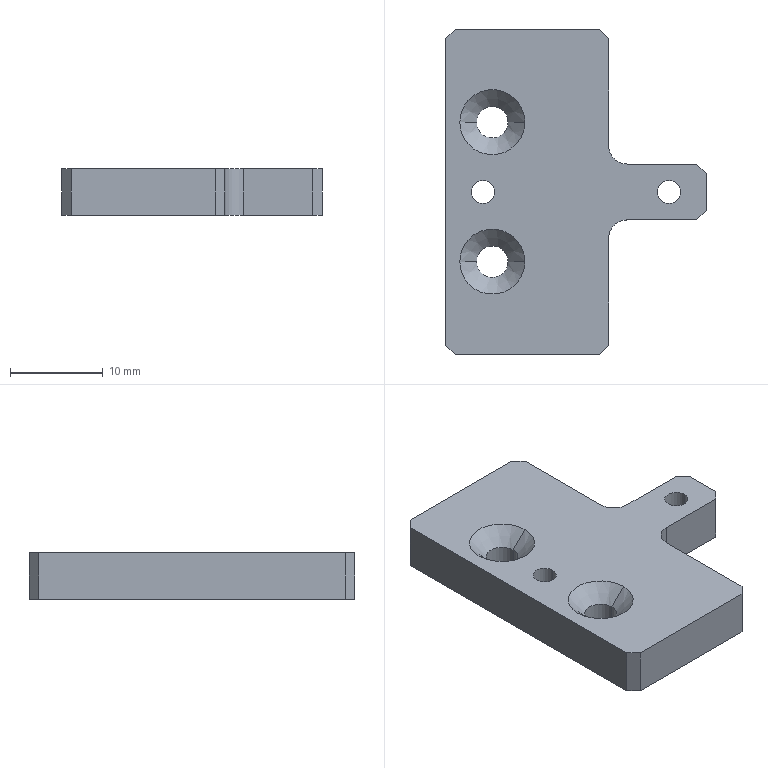Part | NX | features BREP 1 | 1 solid | 30 faces | box 28 x 35 x 5 mm | volume 3184 mm3 | plane 16 | cylinder 10 | cone 4 | commonest cylinder face diameters 2.5 x4 3.4 x4 4 x2
STEP:
#1=CARTESIAN_POINT('',(3.5,5.,0.));
#2=VERTEX_POINT('',#1);
#3=CARTESIAN_POINT('',(5.5,3.,0.));
#4=VERTEX_POINT('',#3);
#5=CARTESIAN_POINT('',(5.5,5.,0.));
#6=DIRECTION('',(0.,0.,1.));
#7=DIRECTION('',(-1.,0.,0.));
#8=AXIS2_PLACEMENT_3D('',#5,#6,#7);
#9=CIRCLE('',#8,2.);
#10=EDGE_CURVE('',#2,#4,#9,.T.);
#11=ORIENTED_EDGE('',*,*,#10,.F.);
#12=CARTESIAN_POINT('',(3.5,5.,5.));
#13=VERTEX_POINT('',#12);
#14=CARTESIAN_POINT('',(3.5,5.,0.));
#15=DIRECTION('',(0.,0.,-1.));
#16=VECTOR('',#15,1000.);
#17=LINE('',#14,#16);
#18=EDGE_CURVE('',#13,#2,#17,.T.);
#19=ORIENTED_EDGE('',*,*,#18,.F.);
#20=CARTESIAN_POINT('',(5.5,3.,5.));
#21=VERTEX_POINT('',#20);
#22=CARTESIAN_POINT('',(5.5,5.,5.));
#23=DIRECTION('',(0.,0.,-1.));
#24=DIRECTION('',(-1.,0.,0.));
#25=AXIS2_PLACEMENT_3D('',#22,#23,#24);
#26=CIRCLE('',#25,2.);
#27=EDGE_CURVE('',#21,#13,#26,.T.);
#28=ORIENTED_EDGE('',*,*,#27,.F.);
#29=CARTESIAN_POINT('',(5.5,3.,5.));
#30=DIRECTION('',(0.,0.,1.));
#31=VECTOR('',#30,1000.);
#32=LINE('',#29,#31);
#33=EDGE_CURVE('',#4,#21,#32,.T.);
#34=ORIENTED_EDGE('',*,*,#33,.F.);
#35=EDGE_LOOP('',(#11,#19,#28,#34));
#36=FACE_BOUND('',#35,.T.);
#37=CARTESIAN_POINT('',(5.5,5.,0.));
#38=DIRECTION('',(0.,0.,-1.));
#39=DIRECTION('',(-1.,0.,0.));
#40=AXIS2_PLACEMENT_3D('',#37,#38,#39);
#41=CYLINDRICAL_SURFACE('',#40,2.);
#42=ADVANCED_FACE('',(#36),#41,.F.);
#43=CARTESIAN_POINT('',(5.5,-3.,0.));
#44=VERTEX_POINT('',#43);
#45=CARTESIAN_POINT('',(3.5,-5.,0.));
#46=VERTEX_POINT('',#45);
#47=CARTESIAN_POINT('',(5.5,-5.,0.));
#48=DIRECTION('',(0.,0.,1.));
#49=DIRECTION('',(-1.,0.,0.));
#50=AXIS2_PLACEMENT_3D('',#47,#48,#49);
#51=CIRCLE('',#50,2.);
#52=EDGE_CURVE('',#44,#46,#51,.T.);
#53=ORIENTED_EDGE('',*,*,#52,.F.);
#54=CARTESIAN_POINT('',(5.5,-3.,5.));
#55=VERTEX_POINT('',#54);
#56=CARTESIAN_POINT('',(5.5,-3.,0.));
#57=DIRECTION('',(0.,0.,-1.));
#58=VECTOR('',#57,1000.);
#59=LINE('',#56,#58);
#60=EDGE_CURVE('',#55,#44,#59,.T.);
#61=ORIENTED_EDGE('',*,*,#60,.F.);
#62=CARTESIAN_POINT('',(3.5,-5.,5.));
#63=VERTEX_POINT('',#62);
#64=CARTESIAN_POINT('',(5.5,-5.,5.));
#65=DIRECTION('',(0.,0.,-1.));
#66=DIRECTION('',(-1.,0.,0.));
#67=AXIS2_PLACEMENT_3D('',#64,#65,#66);
#68=CIRCLE('',#67,2.);
#69=EDGE_CURVE('',#63,#55,#68,.T.);
#70=ORIENTED_EDGE('',*,*,#69,.F.);
#71=CARTESIAN_POINT('',(3.5,-5.,5.));
#72=DIRECTION('',(0.,0.,1.));
#73=VECTOR('',#72,1000.);
#74=LINE('',#71,#73);
#75=EDGE_CURVE('',#46,#63,#74,.T.);
#76=ORIENTED_EDGE('',*,*,#75,.F.);
#77=EDGE_LOOP('',(#53,#61,#70,#76));
#78=FACE_BOUND('',#77,.T.);
#79=CARTESIAN_POINT('',(5.5,-5.,0.));
#80=DIRECTION('',(0.,0.,-1.));
#81=DIRECTION('',(-1.,0.,0.));
#82=AXIS2_PLACEMENT_3D('',#79,#80,#81);
#83=CYLINDRICAL_SURFACE('',#82,2.);
#84=ADVANCED_FACE('',(#78),#83,.F.);
#85=CARTESIAN_POINT('',(3.5,-16.5,0.));
#86=VERTEX_POINT('',#85);
#87=CARTESIAN_POINT('',(2.5,-17.5,0.));
#88=VERTEX_POINT('',#87);
#89=CARTESIAN_POINT('',(10.,-10.,0.));
#90=DIRECTION('',(-0.7071,-0.7071,0.));
#91=VECTOR('',#90,1000.);
#92=LINE('',#89,#91);
#93=EDGE_CURVE('',#86,#88,#92,.T.);
#94=ORIENTED_EDGE('',*,*,#93,.F.);
#95=CARTESIAN_POINT('',(3.5,-16.5,5.));
#96=VERTEX_POINT('',#95);
#97=CARTESIAN_POINT('',(3.5,-16.5,0.));
#98=DIRECTION('',(0.,0.,-1.));
#99=VECTOR('',#98,1000.);
#100=LINE('',#97,#99);
#101=EDGE_CURVE('',#96,#86,#100,.T.);
#102=ORIENTED_EDGE('',*,*,#101,.F.);
#103=CARTESIAN_POINT('',(2.5,-17.5,5.));
#104=VERTEX_POINT('',#103);
#105=CARTESIAN_POINT('',(2.5,-17.5,5.));
#106=DIRECTION('',(0.7071,0.7071,0.));
#107=VECTOR('',#106,1000.);
#108=LINE('',#105,#107);
#109=EDGE_CURVE('',#104,#96,#108,.T.);
#110=ORIENTED_EDGE('',*,*,#109,.F.);
#111=CARTESIAN_POINT('',(2.5,-17.5,5.));
#112=DIRECTION('',(0.,0.,1.));
#113=VECTOR('',#112,1000.);
#114=LINE('',#111,#113);
#115=EDGE_CURVE('',#88,#104,#114,.T.);
#116=ORIENTED_EDGE('',*,*,#115,.F.);
#117=EDGE_LOOP('',(#94,#102,#110,#116));
#118=FACE_BOUND('',#117,.T.);
#119=CARTESIAN_POINT('',(2.5,-17.5,5.));
#120=DIRECTION('',(-0.7071,0.7071,0.));
#121=DIRECTION('',(0.,0.,1.));
#122=AXIS2_PLACEMENT_3D('',#119,#120,#121);
#123=PLANE('',#122);
#124=ADVANCED_FACE('',(#118),#123,.F.);
#125=CARTESIAN_POINT('',(-14.,-16.5,5.));
#126=VERTEX_POINT('',#125);
#127=CARTESIAN_POINT('',(-13.,-17.5,5.));
#128=VERTEX_POINT('',#127);
#129=CARTESIAN_POINT('',(-13.,-17.5,5.));
#130=DIRECTION('',(0.7071,-0.7071,0.));
#131=VECTOR('',#130,1000.);
#132=LINE('',#129,#131);
#133=EDGE_CURVE('',#126,#128,#132,.T.);
#134=ORIENTED_EDGE('',*,*,#133,.F.);
#135=CARTESIAN_POINT('',(-14.,-16.5,0.));
#136=VERTEX_POINT('',#135);
#137=CARTESIAN_POINT('',(-14.,-16.5,5.));
#138=DIRECTION('',(0.,0.,1.));
#139=VECTOR('',#138,1000.);
#140=LINE('',#137,#139);
#141=EDGE_CURVE('',#136,#126,#140,.T.);
#142=ORIENTED_EDGE('',*,*,#141,.F.);
#143=CARTESIAN_POINT('',(-13.,-17.5,0.));
#144=VERTEX_POINT('',#143);
#145=CARTESIAN_POINT('',(-15.25,-15.25,0.));
#146=DIRECTION('',(-0.7071,0.7071,0.));
#147=VECTOR('',#146,1000.);
#148=LINE('',#145,#147);
#149=EDGE_CURVE('',#144,#136,#148,.T.);
#150=ORIENTED_EDGE('',*,*,#149,.F.);
#151=CARTESIAN_POINT('',(-13.,-17.5,5.));
#152=DIRECTION('',(0.,0.,-1.));
#153=VECTOR('',#152,1000.);
#154=LINE('',#151,#153);
#155=EDGE_CURVE('',#128,#144,#154,.T.);
#156=ORIENTED_EDGE('',*,*,#155,.F.);
#157=EDGE_LOOP('',(#134,#142,#150,#156));
#158=FACE_BOUND('',#157,.T.);
#159=CARTESIAN_POINT('',(-13.,-17.5,5.));
#160=DIRECTION('',(0.7071,0.7071,0.));
#161=DIRECTION('',(0.,0.,-1.));
#162=AXIS2_PLACEMENT_3D('',#159,#160,#161);
#163=PLANE('',#162);
#164=ADVANCED_FACE('',(#158),#163,.F.);
#165=CARTESIAN_POINT('',(-13.,17.5,5.));
#166=VERTEX_POINT('',#165);
#167=CARTESIAN_POINT('',(-14.,16.5,5.));
#168=VERTEX_POINT('',#167);
#169=CARTESIAN_POINT('',(-14.,16.5,5.));
#170=DIRECTION('',(-0.7071,-0.7071,0.));
#171=VECTOR('',#170,1000.);
#172=LINE('',#169,#171);
#173=EDGE_CURVE('',#166,#168,#172,.T.);
#174=ORIENTED_EDGE('',*,*,#173,.F.);
#175=CARTESIAN_POINT('',(-13.,17.5,0.));
#176=VERTEX_POINT('',#175);
#177=CARTESIAN_POINT('',(-13.,17.5,5.));
#178=DIRECTION('',(0.,0.,1.));
#179=VECTOR('',#178,1000.);
#180=LINE('',#177,#179);
#181=EDGE_CURVE('',#176,#166,#180,.T.);
#182=ORIENTED_EDGE('',*,*,#181,.F.);
#183=CARTESIAN_POINT('',(-14.,16.5,0.));
#184=VERTEX_POINT('',#183);
#185=CARTESIAN_POINT('',(-15.25,15.25,0.));
#186=DIRECTION('',(0.7071,0.7071,0.));
#187=VECTOR('',#186,1000.);
#188=LINE('',#185,#187);
#189=EDGE_CURVE('',#184,#176,#188,.T.);
#190=ORIENTED_EDGE('',*,*,#189,.F.);
#191=CARTESIAN_POINT('',(-14.,16.5,5.));
#192=DIRECTION('',(0.,0.,-1.));
#193=VECTOR('',#192,1000.);
#194=LINE('',#191,#193);
#195=EDGE_CURVE('',#168,#184,#194,.T.);
#196=ORIENTED_EDGE('',*,*,#195,.F.);
#197=EDGE_LOOP('',(#174,#182,#190,#196));
#198=FACE_BOUND('',#197,.T.);
#199=CARTESIAN_POINT('',(-14.,16.5,5.));
#200=DIRECTION('',(0.7071,-0.7071,0.));
#201=DIRECTION('',(0.,0.,-1.));
#202=AXIS2_PLACEMENT_3D('',#199,#200,#201);
#203=PLANE('',#202);
#204=ADVANCED_FACE('',(#198),#203,.F.);
#205=CARTESIAN_POINT('',(2.5,17.5,0.));
#206=VERTEX_POINT('',#205);
#207=CARTESIAN_POINT('',(3.5,16.5,0.));
#208=VERTEX_POINT('',#207);
#209=CARTESIAN_POINT('',(10.,10.,0.));
#210=DIRECTION('',(0.7071,-0.7071,0.));
#211=VECTOR('',#210,1000.);
#212=LINE('',#209,#211);
#213=EDGE_CURVE('',#206,#208,#212,.T.);
#214=ORIENTED_EDGE('',*,*,#213,.F.);
#215=CARTESIAN_POINT('',(2.5,17.5,5.));
#216=VERTEX_POINT('',#215);
#217=CARTESIAN_POINT('',(2.5,17.5,5.));
#218=DIRECTION('',(0.,0.,-1.));
#219=VECTOR('',#218,1000.);
#220=LINE('',#217,#219);
#221=EDGE_CURVE('',#216,#206,#220,.T.);
#222=ORIENTED_EDGE('',*,*,#221,.F.);
#223=CARTESIAN_POINT('',(3.5,16.5,5.));
#224=VERTEX_POINT('',#223);
#225=CARTESIAN_POINT('',(3.5,16.5,5.));
#226=DIRECTION('',(-0.7071,0.7071,0.));
#227=VECTOR('',#226,1000.);
#228=LINE('',#225,#227);
#229=EDGE_CURVE('',#224,#216,#228,.T.);
#230=ORIENTED_EDGE('',*,*,#229,.F.);
#231=CARTESIAN_POINT('',(3.5,16.5,0.));
#232=DIRECTION('',(0.,0.,1.));
#233=VECTOR('',#232,1000.);
#234=LINE('',#231,#233);
#235=EDGE_CURVE('',#208,#224,#234,.T.);
#236=ORIENTED_EDGE('',*,*,#235,.F.);
#237=EDGE_LOOP('',(#214,#222,#230,#236));
#238=FACE_BOUND('',#237,.T.);
#239=CARTESIAN_POINT('',(3.5,16.5,0.));
#240=DIRECTION('',(-0.7071,-0.7071,0.));
#241=DIRECTION('',(0.,0.,1.));
#242=AXIS2_PLACEMENT_3D('',#239,#240,#241);
#243=PLANE('',#242);
#244=ADVANCED_FACE('',(#238),#243,.F.);
#245=CARTESIAN_POINT('',(14.,-2.,0.));
#246=VERTEX_POINT('',#245);
#247=CARTESIAN_POINT('',(13.,-3.,0.));
#248=VERTEX_POINT('',#247);
#249=CARTESIAN_POINT('',(8.,-8.,0.));
#250=DIRECTION('',(-0.7071,-0.7071,0.));
#251=VECTOR('',#250,1000.);
#252=LINE('',#249,#251);
#253=EDGE_CURVE('',#246,#248,#252,.T.);
#254=ORIENTED_EDGE('',*,*,#253,.F.);
#255=CARTESIAN_POINT('',(14.,-2.,5.));
#256=VERTEX_POINT('',#255);
#257=CARTESIAN_POINT('',(14.,-2.,5.));
#258=DIRECTION('',(0.,0.,-1.));
#259=VECTOR('',#258,1000.);
#260=LINE('',#257,#259);
#261=EDGE_CURVE('',#256,#246,#260,.T.);
#262=ORIENTED_EDGE('',*,*,#261,.F.);
#263=CARTESIAN_POINT('',(13.,-3.,5.));
#264=VERTEX_POINT('',#263);
#265=CARTESIAN_POINT('',(13.,-3.,5.));
#266=DIRECTION('',(0.7071,0.7071,0.));
#267=VECTOR('',#266,1000.);
#268=LINE('',#265,#267);
#269=EDGE_CURVE('',#264,#256,#268,.T.);
#270=ORIENTED_EDGE('',*,*,#269,.F.);
#271=CARTESIAN_POINT('',(13.,-3.,0.));
#272=DIRECTION('',(0.,0.,1.));
#273=VECTOR('',#272,1000.);
#274=LINE('',#271,#273);
#275=EDGE_CURVE('',#248,#264,#274,.T.);
#276=ORIENTED_EDGE('',*,*,#275,.F.);
#277=EDGE_LOOP('',(#254,#262,#270,#276));
#278=FACE_BOUND('',#277,.T.);
#279=CARTESIAN_POINT('',(13.,-3.,0.));
#280=DIRECTION('',(-0.7071,0.7071,0.));
#281=DIRECTION('',(0.,0.,1.));
#282=AXIS2_PLACEMENT_3D('',#279,#280,#281);
#283=PLANE('',#282);
#284=ADVANCED_FACE('',(#278),#283,.F.);
#285=CARTESIAN_POINT('',(13.,3.,0.));
#286=VERTEX_POINT('',#285);
#287=CARTESIAN_POINT('',(14.,2.,0.));
#288=VERTEX_POINT('',#287);
#289=CARTESIAN_POINT('',(8.,8.,0.));
#290=DIRECTION('',(0.7071,-0.7071,0.));
#291=VECTOR('',#290,1000.);
#292=LINE('',#289,#291);
#293=EDGE_CURVE('',#286,#288,#292,.T.);
#294=ORIENTED_EDGE('',*,*,#293,.F.);
#295=CARTESIAN_POINT('',(13.,3.,5.));
#296=VERTEX_POINT('',#295);
#297=CARTESIAN_POINT('',(13.,3.,0.));
#298=DIRECTION('',(0.,0.,-1.));
#299=VECTOR('',#298,1000.);
#300=LINE('',#297,#299);
#301=EDGE_CURVE('',#296,#286,#300,.T.);
#302=ORIENTED_EDGE('',*,*,#301,.F.);
#303=CARTESIAN_POINT('',(14.,2.,5.));
#304=VERTEX_POINT('',#303);
#305=CARTESIAN_POINT('',(14.,2.,5.));
#306=DIRECTION('',(-0.7071,0.7071,0.));
#307=VECTOR('',#306,1000.);
#308=LINE('',#305,#307);
#309=EDGE_CURVE('',#304,#296,#308,.T.);
#310=ORIENTED_EDGE('',*,*,#309,.F.);
#311=CARTESIAN_POINT('',(14.,2.,5.));
#312=DIRECTION('',(0.,0.,1.));
#313=VECTOR('',#312,1000.);
#314=LINE('',#311,#313);
#315=EDGE_CURVE('',#288,#304,#314,.T.);
#316=ORIENTED_EDGE('',*,*,#315,.F.);
#317=EDGE_LOOP('',(#294,#302,#310,#316));
#318=FACE_BOUND('',#317,.T.);
#319=CARTESIAN_POINT('',(14.,2.,5.));
#320=DIRECTION('',(-0.7071,-0.7071,0.));
#321=DIRECTION('',(0.,0.,1.));
#322=AXIS2_PLACEMENT_3D('',#319,#320,#321);
#323=PLANE('',#322);
#324=ADVANCED_FACE('',(#318),#323,.F.);
#325=CARTESIAN_POINT('',(14.,-3.,5.));
#326=DIRECTION('',(-1.,0.,0.));
#327=VECTOR('',#326,1000.);
#328=LINE('',#325,#327);
#329=EDGE_CURVE('',#264,#55,#328,.T.);
#330=ORIENTED_EDGE('',*,*,#329,.T.);
#331=ORIENTED_EDGE('',*,*,#60,.T.);
#332=CARTESIAN_POINT('',(14.,-3.,0.));
#333=DIRECTION('',(-1.,0.,0.));
#334=VECTOR('',#333,1000.);
#335=LINE('',#332,#334);
#336=EDGE_CURVE('',#248,#44,#335,.T.);
#337=ORIENTED_EDGE('',*,*,#336,.F.);
#338=ORIENTED_EDGE('',*,*,#275,.T.);
#339=EDGE_LOOP('',(#330,#331,#337,#338));
#340=FACE_BOUND('',#339,.T.);
#341=CARTESIAN_POINT('',(14.,-3.,0.));
#342=DIRECTION('',(0.,1.,0.));
#343=DIRECTION('',(-1.,0.,0.));
#344=AXIS2_PLACEMENT_3D('',#341,#342,#343);
#345=PLANE('',#344);
#346=ADVANCED_FACE('',(#340),#345,.F.);
#347=CARTESIAN_POINT('',(3.5,-17.5,0.));
#348=DIRECTION('',(0.,-1.,0.));
#349=VECTOR('',#348,1000.);
#350=LINE('',#347,#349);
#351=EDGE_CURVE('',#46,#86,#350,.T.);
#352=ORIENTED_EDGE('',*,*,#351,.F.);
#353=ORIENTED_EDGE('',*,*,#75,.T.);
#354=CARTESIAN_POINT('',(3.5,-17.5,5.));
#355=DIRECTION('',(0.,-1.,0.));
#356=VECTOR('',#355,1000.);
#357=LINE('',#354,#356);
#358=EDGE_CURVE('',#63,#96,#357,.T.);
#359=ORIENTED_EDGE('',*,*,#358,.T.);
#360=ORIENTED_EDGE('',*,*,#101,.T.);
#361=EDGE_LOOP('',(#352,#353,#359,#360));
#362=FACE_BOUND('',#361,.T.);
#363=CARTESIAN_POINT('',(3.5,-17.5,0.));
#364=DIRECTION('',(-1.,0.,0.));
#365=DIRECTION('',(0.,0.,1.));
#366=AXIS2_PLACEMENT_3D('',#363,#364,#365);
#367=PLANE('',#366);
#368=ADVANCED_FACE('',(#362),#367,.F.);
#369=CARTESIAN_POINT('',(3.5,17.5,5.));
#370=DIRECTION('',(0.,-1.,0.));
#371=VECTOR('',#370,1000.);
#372=LINE('',#369,#371);
#373=EDGE_CURVE('',#224,#13,#372,.T.);
#374=ORIENTED_EDGE('',*,*,#373,.T.);
#375=ORIENTED_EDGE('',*,*,#18,.T.);
#376=CARTESIAN_POINT('',(3.5,17.5,0.));
#377=DIRECTION('',(0.,-1.,0.));
#378=VECTOR('',#377,1000.);
#379=LINE('',#376,#378);
#380=EDGE_CURVE('',#208,#2,#379,.T.);
#381=ORIENTED_EDGE('',*,*,#380,.F.);
#382=ORIENTED_EDGE('',*,*,#235,.T.);
#383=EDGE_LOOP('',(#374,#375,#381,#382));
#384=FACE_BOUND('',#383,.T.);
#385=CARTESIAN_POINT('',(3.5,17.5,0.));
#386=DIRECTION('',(-1.,0.,0.));
#387=DIRECTION('',(0.,-1.,0.));
#388=AXIS2_PLACEMENT_3D('',#385,#386,#387);
#389=PLANE('',#388);
#390=ADVANCED_FACE('',(#384),#389,.F.);
#391=CARTESIAN_POINT('',(14.,3.,0.));
#392=DIRECTION('',(1.,0.,0.));
#393=VECTOR('',#392,1000.);
#394=LINE('',#391,#393);
#395=EDGE_CURVE('',#4,#286,#394,.T.);
#396=ORIENTED_EDGE('',*,*,#395,.F.);
#397=ORIENTED_EDGE('',*,*,#33,.T.);
#398=CARTESIAN_POINT('',(14.,3.,5.));
#399=DIRECTION('',(1.,0.,0.));
#400=VECTOR('',#399,1000.);
#401=LINE('',#398,#400);
#402=EDGE_CURVE('',#21,#296,#401,.T.);
#403=ORIENTED_EDGE('',*,*,#402,.T.);
#404=ORIENTED_EDGE('',*,*,#301,.T.);
#405=EDGE_LOOP('',(#396,#397,#403,#404));
#406=FACE_BOUND('',#405,.T.);
#407=CARTESIAN_POINT('',(14.,3.,0.));
#408=DIRECTION('',(0.,-1.,0.));
#409=DIRECTION('',(1.,0.,0.));
#410=AXIS2_PLACEMENT_3D('',#407,#408,#409);
#411=PLANE('',#410);
#412=ADVANCED_FACE('',(#406),#411,.F.);
#413=CARTESIAN_POINT('',(-12.5,7.5,5.));
#414=VERTEX_POINT('',#413);
#415=CARTESIAN_POINT('',(-10.7,7.5,3.2));
#416=VERTEX_POINT('',#415);
#417=CARTESIAN_POINT('',(-12.5,7.5,5.));
#418=DIRECTION('',(-0.7071,0.,0.7071));
#419=VECTOR('',#418,1000.);
#420=LINE('',#417,#419);
#421=EDGE_CURVE('',#414,#416,#420,.F.);
#422=ORIENTED_EDGE('',*,*,#421,.T.);
#423=CARTESIAN_POINT('',(-7.3,7.5,3.2));
#424=VERTEX_POINT('',#423);
#425=CARTESIAN_POINT('',(-9.,7.5,3.2));
#426=DIRECTION('',(0.,0.,1.));
#427=DIRECTION('',(1.,0.,0.));
#428=AXIS2_PLACEMENT_3D('',#425,#426,#427);
#429=CIRCLE('',#428,1.7);
#430=EDGE_CURVE('',#424,#416,#429,.T.);
#431=ORIENTED_EDGE('',*,*,#430,.F.);
#432=CARTESIAN_POINT('',(-5.5,7.5,5.));
#433=VERTEX_POINT('',#432);
#434=CARTESIAN_POINT('',(-5.5,7.5,5.));
#435=DIRECTION('',(0.7071,0.,0.7071));
#436=VECTOR('',#435,1000.);
#437=LINE('',#434,#436);
#438=EDGE_CURVE('',#433,#424,#437,.F.);
#439=ORIENTED_EDGE('',*,*,#438,.F.);
#440=CARTESIAN_POINT('',(-9.,7.5,5.));
#441=DIRECTION('',(0.,0.,1.));
#442=DIRECTION('',(1.,0.,0.));
#443=AXIS2_PLACEMENT_3D('',#440,#441,#442);
#444=CIRCLE('',#443,3.5);
#445=EDGE_CURVE('',#433,#414,#444,.T.);
#446=ORIENTED_EDGE('',*,*,#445,.T.);
#447=EDGE_LOOP('',(#422,#431,#439,#446));
#448=FACE_BOUND('',#447,.T.);
#449=CARTESIAN_POINT('',(-9.,7.5,5.));
#450=DIRECTION('',(0.,0.,1.));
#451=DIRECTION('',(1.,0.,0.));
#452=AXIS2_PLACEMENT_3D('',#449,#450,#451);
#453=CONICAL_SURFACE('',#452,3.5,0.7854);
#454=ADVANCED_FACE('',(#448),#453,.F.);
#455=CARTESIAN_POINT('',(-10.7,7.5,0.));
#456=VERTEX_POINT('',#455);
#457=CARTESIAN_POINT('',(-10.7,7.5,5.));
#458=DIRECTION('',(0.,0.,1.));
#459=VECTOR('',#458,1000.);
#460=LINE('',#457,#459);
#461=EDGE_CURVE('',#416,#456,#460,.F.);
#462=ORIENTED_EDGE('',*,*,#461,.T.);
#463=CARTESIAN_POINT('',(-7.3,7.5,0.));
#464=VERTEX_POINT('',#463);
#465=CARTESIAN_POINT('',(-9.,7.5,0.));
#466=DIRECTION('',(0.,0.,-1.));
#467=DIRECTION('',(-1.,0.,0.));
#468=AXIS2_PLACEMENT_3D('',#465,#466,#467);
#469=CIRCLE('',#468,1.7);
#470=EDGE_CURVE('',#456,#464,#469,.T.);
#471=ORIENTED_EDGE('',*,*,#470,.T.);
#472=CARTESIAN_POINT('',(-7.3,7.5,5.));
#473=DIRECTION('',(0.,0.,1.));
#474=VECTOR('',#473,1000.);
#475=LINE('',#472,#474);
#476=EDGE_CURVE('',#424,#464,#475,.F.);
#477=ORIENTED_EDGE('',*,*,#476,.F.);
#478=ORIENTED_EDGE('',*,*,#430,.T.);
#479=EDGE_LOOP('',(#462,#471,#477,#478));
#480=FACE_BOUND('',#479,.T.);
#481=CARTESIAN_POINT('',(-9.,7.5,5.));
#482=DIRECTION('',(0.,0.,1.));
#483=DIRECTION('',(1.,0.,0.));
#484=AXIS2_PLACEMENT_3D('',#481,#482,#483);
#485=CYLINDRICAL_SURFACE('',#484,1.7);
#486=ADVANCED_FACE('',(#480),#485,.F.);
#487=CARTESIAN_POINT('',(-12.5,-7.5,5.));
#488=VERTEX_POINT('',#487);
#489=CARTESIAN_POINT('',(-10.7,-7.5,3.2));
#490=VERTEX_POINT('',#489);
#491=CARTESIAN_POINT('',(-12.5,-7.5,5.));
#492=DIRECTION('',(-0.7071,0.,0.7071));
#493=VECTOR('',#492,1000.);
#494=LINE('',#491,#493);
#495=EDGE_CURVE('',#488,#490,#494,.F.);
#496=ORIENTED_EDGE('',*,*,#495,.T.);
#497=CARTESIAN_POINT('',(-7.3,-7.5,3.2));
#498=VERTEX_POINT('',#497);
#499=CARTESIAN_POINT('',(-9.,-7.5,3.2));
#500=DIRECTION('',(0.,0.,1.));
#501=DIRECTION('',(1.,0.,0.));
#502=AXIS2_PLACEMENT_3D('',#499,#500,#501);
#503=CIRCLE('',#502,1.7);
#504=EDGE_CURVE('',#498,#490,#503,.T.);
#505=ORIENTED_EDGE('',*,*,#504,.F.);
#506=CARTESIAN_POINT('',(-5.5,-7.5,5.));
#507=VERTEX_POINT('',#506);
#508=CARTESIAN_POINT('',(-5.5,-7.5,5.));
#509=DIRECTION('',(0.7071,0.,0.7071));
#510=VECTOR('',#509,1000.);
#511=LINE('',#508,#510);
#512=EDGE_CURVE('',#507,#498,#511,.F.);
#513=ORIENTED_EDGE('',*,*,#512,.F.);
#514=CARTESIAN_POINT('',(-9.,-7.5,5.));
#515=DIRECTION('',(0.,0.,1.));
#516=DIRECTION('',(1.,0.,0.));
#517=AXIS2_PLACEMENT_3D('',#514,#515,#516);
#518=CIRCLE('',#517,3.5);
#519=EDGE_CURVE('',#507,#488,#518,.T.);
#520=ORIENTED_EDGE('',*,*,#519,.T.);
#521=EDGE_LOOP('',(#496,#505,#513,#520));
#522=FACE_BOUND('',#521,.T.);
#523=CARTESIAN_POINT('',(-9.,-7.5,5.));
#524=DIRECTION('',(0.,0.,1.));
#525=DIRECTION('',(1.,0.,0.));
#526=AXIS2_PLACEMENT_3D('',#523,#524,#525);
#527=CONICAL_SURFACE('',#526,3.5,0.7854);
#528=ADVANCED_FACE('',(#522),#527,.F.);
#529=CARTESIAN_POINT('',(-10.7,-7.5,0.));
#530=VERTEX_POINT('',#529);
#531=CARTESIAN_POINT('',(-10.7,-7.5,5.));
#532=DIRECTION('',(0.,0.,1.));
#533=VECTOR('',#532,1000.);
#534=LINE('',#531,#533);
#535=EDGE_CURVE('',#490,#530,#534,.F.);
#536=ORIENTED_EDGE('',*,*,#535,.T.);
#537=CARTESIAN_POINT('',(-7.3,-7.5,0.));
#538=VERTEX_POINT('',#537);
#539=CARTESIAN_POINT('',(-9.,-7.5,0.));
#540=DIRECTION('',(0.,0.,-1.));
#541=DIRECTION('',(-1.,0.,0.));
#542=AXIS2_PLACEMENT_3D('',#539,#540,#541);
#543=CIRCLE('',#542,1.7);
#544=EDGE_CURVE('',#530,#538,#543,.T.);
#545=ORIENTED_EDGE('',*,*,#544,.T.);
#546=CARTESIAN_POINT('',(-7.3,-7.5,5.));
#547=DIRECTION('',(0.,0.,1.));
#548=VECTOR('',#547,1000.);
#549=LINE('',#546,#548);
#550=EDGE_CURVE('',#498,#538,#549,.F.);
#551=ORIENTED_EDGE('',*,*,#550,.F.);
#552=ORIENTED_EDGE('',*,*,#504,.T.);
#553=EDGE_LOOP('',(#536,#545,#551,#552));
#554=FACE_BOUND('',#553,.T.);
#555=CARTESIAN_POINT('',(-9.,-7.5,5.));
#556=DIRECTION('',(0.,0.,1.));
#557=DIRECTION('',(1.,0.,0.));
#558=AXIS2_PLACEMENT_3D('',#555,#556,#557);
#559=CYLINDRICAL_SURFACE('',#558,1.7);
#560=ADVANCED_FACE('',(#554),#559,.F.);
#561=CARTESIAN_POINT('',(8.75,0.,5.));
#562=VERTEX_POINT('',#561);
#563=CARTESIAN_POINT('',(8.75,0.,0.));
#564=VERTEX_POINT('',#563);
#565=CARTESIAN_POINT('',(8.75,0.,5.));
#566=DIRECTION('',(0.,0.,1.));
#567=VECTOR('',#566,1000.);
#568=LINE('',#565,#567);
#569=EDGE_CURVE('',#562,#564,#568,.F.);
#570=ORIENTED_EDGE('',*,*,#569,.T.);
#571=CARTESIAN_POINT('',(11.25,0.,0.));
#572=VERTEX_POINT('',#571);
#573=CARTESIAN_POINT('',(10.,0.,0.));
#574=DIRECTION('',(0.,0.,-1.));
#575=DIRECTION('',(-1.,0.,0.));
#576=AXIS2_PLACEMENT_3D('',#573,#574,#575);
#577=CIRCLE('',#576,1.25);
#578=EDGE_CURVE('',#564,#572,#577,.T.);
#579=ORIENTED_EDGE('',*,*,#578,.T.);
#580=CARTESIAN_POINT('',(11.25,0.,5.));
#581=VERTEX_POINT('',#580);
#582=CARTESIAN_POINT('',(11.25,0.,5.));
#583=DIRECTION('',(0.,0.,1.));
#584=VECTOR('',#583,1000.);
#585=LINE('',#582,#584);
#586=EDGE_CURVE('',#581,#572,#585,.F.);
#587=ORIENTED_EDGE('',*,*,#586,.F.);
#588=CARTESIAN_POINT('',(10.,0.,5.));
#589=DIRECTION('',(0.,0.,1.));
#590=DIRECTION('',(1.,0.,0.));
#591=AXIS2_PLACEMENT_3D('',#588,#589,#590);
#592=CIRCLE('',#591,1.25);
#593=EDGE_CURVE('',#581,#562,#592,.T.);
#594=ORIENTED_EDGE('',*,*,#593,.T.);
#595=EDGE_LOOP('',(#570,#579,#587,#594));
#596=FACE_BOUND('',#595,.T.);
#597=CARTESIAN_POINT('',(10.,0.,5.));
#598=DIRECTION('',(0.,0.,1.));
#599=DIRECTION('',(1.,0.,0.));
#600=AXIS2_PLACEMENT_3D('',#597,#598,#599);
#601=CYLINDRICAL_SURFACE('',#600,1.25);
#602=ADVANCED_FACE('',(#596),#601,.F.);
#603=CARTESIAN_POINT('',(-11.25,0.,5.));
#604=VERTEX_POINT('',#603);
#605=CARTESIAN_POINT('',(-11.25,0.,0.));
#606=VERTEX_POINT('',#605);
#607=CARTESIAN_POINT('',(-11.25,0.,5.));
#608=DIRECTION('',(0.,0.,1.));
#609=VECTOR('',#608,1000.);
#610=LINE('',#607,#609);
#611=EDGE_CURVE('',#604,#606,#610,.F.);
#612=ORIENTED_EDGE('',*,*,#611,.T.);
#613=CARTESIAN_POINT('',(-8.75,0.,0.));
#614=VERTEX_POINT('',#613);
#615=CARTESIAN_POINT('',(-10.,0.,0.));
#616=DIRECTION('',(0.,0.,-1.));
#617=DIRECTION('',(-1.,0.,0.));
#618=AXIS2_PLACEMENT_3D('',#615,#616,#617);
#619=CIRCLE('',#618,1.25);
#620=EDGE_CURVE('',#606,#614,#619,.T.);
#621=ORIENTED_EDGE('',*,*,#620,.T.);
#622=CARTESIAN_POINT('',(-8.75,0.,5.));
#623=VERTEX_POINT('',#622);
#624=CARTESIAN_POINT('',(-8.75,0.,5.));
#625=DIRECTION('',(0.,0.,1.));
#626=VECTOR('',#625,1000.);
#627=LINE('',#624,#626);
#628=EDGE_CURVE('',#623,#614,#627,.F.);
#629=ORIENTED_EDGE('',*,*,#628,.F.);
#630=CARTESIAN_POINT('',(-10.,0.,5.));
#631=DIRECTION('',(0.,0.,1.));
#632=DIRECTION('',(1.,0.,0.));
#633=AXIS2_PLACEMENT_3D('',#630,#631,#632);
#634=CIRCLE('',#633,1.25);
#635=EDGE_CURVE('',#623,#604,#634,.T.);
#636=ORIENTED_EDGE('',*,*,#635,.T.);
#637=EDGE_LOOP('',(#612,#621,#629,#636));
#638=FACE_BOUND('',#637,.T.);
#639=CARTESIAN_POINT('',(-10.,0.,5.));
#640=DIRECTION('',(0.,0.,1.));
#641=DIRECTION('',(1.,0.,0.));
#642=AXIS2_PLACEMENT_3D('',#639,#640,#641);
#643=CYLINDRICAL_SURFACE('',#642,1.25);
#644=ADVANCED_FACE('',(#638),#643,.F.);
#645=CARTESIAN_POINT('',(-10.,0.,0.));
#646=DIRECTION('',(0.,0.,-1.));
#647=DIRECTION('',(-1.,0.,0.));
#648=AXIS2_PLACEMENT_3D('',#645,#646,#647);
#649=CIRCLE('',#648,1.25);
#650=EDGE_CURVE('',#614,#606,#649,.T.);
#651=ORIENTED_EDGE('',*,*,#650,.F.);
#652=ORIENTED_EDGE('',*,*,#620,.F.);
#653=EDGE_LOOP('',(#651,#652));
#654=FACE_BOUND('',#653,.T.);
#655=CARTESIAN_POINT('',(10.,0.,0.));
#656=DIRECTION('',(0.,0.,-1.));
#657=DIRECTION('',(-1.,0.,0.));
#658=AXIS2_PLACEMENT_3D('',#655,#656,#657);
#659=CIRCLE('',#658,1.25);
#660=EDGE_CURVE('',#572,#564,#659,.T.);
#661=ORIENTED_EDGE('',*,*,#660,.F.);
#662=ORIENTED_EDGE('',*,*,#578,.F.);
#663=EDGE_LOOP('',(#661,#662));
#664=FACE_BOUND('',#663,.T.);
#665=CARTESIAN_POINT('',(-9.,-7.5,0.));
#666=DIRECTION('',(0.,0.,-1.));
#667=DIRECTION('',(-1.,0.,0.));
#668=AXIS2_PLACEMENT_3D('',#665,#666,#667);
#669=CIRCLE('',#668,1.7);
#670=EDGE_CURVE('',#538,#530,#669,.T.);
#671=ORIENTED_EDGE('',*,*,#670,.F.);
#672=ORIENTED_EDGE('',*,*,#544,.F.);
#673=EDGE_LOOP('',(#671,#672));
#674=FACE_BOUND('',#673,.T.);
#675=CARTESIAN_POINT('',(-9.,7.5,0.));
#676=DIRECTION('',(0.,0.,-1.));
#677=DIRECTION('',(-1.,0.,0.));
#678=AXIS2_PLACEMENT_3D('',#675,#676,#677);
#679=CIRCLE('',#678,1.7);
#680=EDGE_CURVE('',#464,#456,#679,.T.);
#681=ORIENTED_EDGE('',*,*,#680,.F.);
#682=ORIENTED_EDGE('',*,*,#470,.F.);
#683=EDGE_LOOP('',(#681,#682));
#684=FACE_BOUND('',#683,.T.);
#685=CARTESIAN_POINT('',(-14.,17.5,0.));
#686=DIRECTION('',(-1.,0.,0.));
#687=VECTOR('',#686,1000.);
#688=LINE('',#685,#687);
#689=EDGE_CURVE('',#206,#176,#688,.T.);
#690=ORIENTED_EDGE('',*,*,#689,.F.);
#691=ORIENTED_EDGE('',*,*,#213,.T.);
#692=ORIENTED_EDGE('',*,*,#380,.T.);
#693=ORIENTED_EDGE('',*,*,#10,.T.);
#694=ORIENTED_EDGE('',*,*,#395,.T.);
#695=ORIENTED_EDGE('',*,*,#293,.T.);
#696=CARTESIAN_POINT('',(14.,-17.5,0.));
#697=DIRECTION('',(0.,1.,0.));
#698=VECTOR('',#697,1000.);
#699=LINE('',#696,#698);
#700=EDGE_CURVE('',#246,#288,#699,.T.);
#701=ORIENTED_EDGE('',*,*,#700,.F.);
#702=ORIENTED_EDGE('',*,*,#253,.T.);
#703=ORIENTED_EDGE('',*,*,#336,.T.);
#704=ORIENTED_EDGE('',*,*,#52,.T.);
#705=ORIENTED_EDGE('',*,*,#351,.T.);
#706=ORIENTED_EDGE('',*,*,#93,.T.);
#707=CARTESIAN_POINT('',(-14.,-17.5,0.));
#708=DIRECTION('',(1.,0.,0.));
#709=VECTOR('',#708,1000.);
#710=LINE('',#707,#709);
#711=EDGE_CURVE('',#144,#88,#710,.T.);
#712=ORIENTED_EDGE('',*,*,#711,.F.);
#713=ORIENTED_EDGE('',*,*,#149,.T.);
#714=CARTESIAN_POINT('',(-14.,-17.5,0.));
#715=DIRECTION('',(0.,-1.,0.));
#716=VECTOR('',#715,1000.);
#717=LINE('',#714,#716);
#718=EDGE_CURVE('',#184,#136,#717,.T.);
#719=ORIENTED_EDGE('',*,*,#718,.F.);
#720=ORIENTED_EDGE('',*,*,#189,.T.);
#721=EDGE_LOOP('',(#690,#691,#692,#693,#694,#695,#701,#702,#703,#704,#705,#706,#712,#713,#719,#720));
#722=FACE_BOUND('',#721,.T.);
#723=CARTESIAN_POINT('',(0.,0.,0.));
#724=DIRECTION('',(0.,0.,-1.));
#725=DIRECTION('',(-1.,0.,0.));
#726=AXIS2_PLACEMENT_3D('',#723,#724,#725);
#727=PLANE('',#726);
#728=ADVANCED_FACE('',(#654,#664,#674,#684,#722),#727,.T.);
#729=ORIENTED_EDGE('',*,*,#373,.F.);
#730=ORIENTED_EDGE('',*,*,#229,.T.);
#731=CARTESIAN_POINT('',(-14.,17.5,5.));
#732=DIRECTION('',(-1.,0.,0.));
#733=VECTOR('',#732,1000.);
#734=LINE('',#731,#733);
#735=EDGE_CURVE('',#216,#166,#734,.T.);
#736=ORIENTED_EDGE('',*,*,#735,.T.);
#737=ORIENTED_EDGE('',*,*,#173,.T.);
#738=CARTESIAN_POINT('',(-14.,-17.5,5.));
#739=DIRECTION('',(0.,-1.,0.));
#740=VECTOR('',#739,1000.);
#741=LINE('',#738,#740);
#742=EDGE_CURVE('',#168,#126,#741,.T.);
#743=ORIENTED_EDGE('',*,*,#742,.T.);
#744=ORIENTED_EDGE('',*,*,#133,.T.);
#745=CARTESIAN_POINT('',(-14.,-17.5,5.));
#746=DIRECTION('',(1.,0.,0.));
#747=VECTOR('',#746,1000.);
#748=LINE('',#745,#747);
#749=EDGE_CURVE('',#128,#104,#748,.T.);
#750=ORIENTED_EDGE('',*,*,#749,.T.);
#751=ORIENTED_EDGE('',*,*,#109,.T.);
#752=ORIENTED_EDGE('',*,*,#358,.F.);
#753=ORIENTED_EDGE('',*,*,#69,.T.);
#754=ORIENTED_EDGE('',*,*,#329,.F.);
#755=ORIENTED_EDGE('',*,*,#269,.T.);
#756=CARTESIAN_POINT('',(14.,-17.5,5.));
#757=DIRECTION('',(0.,1.,0.));
#758=VECTOR('',#757,1000.);
#759=LINE('',#756,#758);
#760=EDGE_CURVE('',#256,#304,#759,.T.);
#761=ORIENTED_EDGE('',*,*,#760,.T.);
#762=ORIENTED_EDGE('',*,*,#309,.T.);
#763=ORIENTED_EDGE('',*,*,#402,.F.);
#764=ORIENTED_EDGE('',*,*,#27,.T.);
#765=EDGE_LOOP('',(#729,#730,#736,#737,#743,#744,#750,#751,#752,#753,#754,#755,#761,#762,#763,#764));
#766=FACE_BOUND('',#765,.T.);
#767=ORIENTED_EDGE('',*,*,#635,.F.);
#768=CARTESIAN_POINT('',(-10.,0.,5.));
#769=DIRECTION('',(0.,0.,1.));
#770=DIRECTION('',(1.,0.,0.));
#771=AXIS2_PLACEMENT_3D('',#768,#769,#770);
#772=CIRCLE('',#771,1.25);
#773=EDGE_CURVE('',#604,#623,#772,.T.);
#774=ORIENTED_EDGE('',*,*,#773,.F.);
#775=EDGE_LOOP('',(#767,#774));
#776=FACE_BOUND('',#775,.T.);
#777=ORIENTED_EDGE('',*,*,#593,.F.);
#778=CARTESIAN_POINT('',(10.,0.,5.));
#779=DIRECTION('',(0.,0.,1.));
#780=DIRECTION('',(1.,0.,0.));
#781=AXIS2_PLACEMENT_3D('',#778,#779,#780);
#782=CIRCLE('',#781,1.25);
#783=EDGE_CURVE('',#562,#581,#782,.T.);
#784=ORIENTED_EDGE('',*,*,#783,.F.);
#785=EDGE_LOOP('',(#777,#784));
#786=FACE_BOUND('',#785,.T.);
#787=ORIENTED_EDGE('',*,*,#519,.F.);
#788=CARTESIAN_POINT('',(-9.,-7.5,5.));
#789=DIRECTION('',(0.,0.,1.));
#790=DIRECTION('',(1.,0.,0.));
#791=AXIS2_PLACEMENT_3D('',#788,#789,#790);
#792=CIRCLE('',#791,3.5);
#793=EDGE_CURVE('',#488,#507,#792,.T.);
#794=ORIENTED_EDGE('',*,*,#793,.F.);
#795=EDGE_LOOP('',(#787,#794));
#796=FACE_BOUND('',#795,.T.);
#797=ORIENTED_EDGE('',*,*,#445,.F.);
#798=CARTESIAN_POINT('',(-9.,7.5,5.));
#799=DIRECTION('',(0.,0.,1.));
#800=DIRECTION('',(1.,0.,0.));
#801=AXIS2_PLACEMENT_3D('',#798,#799,#800);
#802=CIRCLE('',#801,3.5);
#803=EDGE_CURVE('',#414,#433,#802,.T.);
#804=ORIENTED_EDGE('',*,*,#803,.F.);
#805=EDGE_LOOP('',(#797,#804));
#806=FACE_BOUND('',#805,.T.);
#807=CARTESIAN_POINT('',(0.,0.,5.));
#808=DIRECTION('',(0.,0.,-1.));
#809=DIRECTION('',(-1.,0.,0.));
#810=AXIS2_PLACEMENT_3D('',#807,#808,#809);
#811=PLANE('',#810);
#812=ADVANCED_FACE('',(#766,#776,#786,#796,#806),#811,.F.);
#813=ORIENTED_EDGE('',*,*,#749,.F.);
#814=ORIENTED_EDGE('',*,*,#155,.T.);
#815=ORIENTED_EDGE('',*,*,#711,.T.);
#816=ORIENTED_EDGE('',*,*,#115,.T.);
#817=EDGE_LOOP('',(#813,#814,#815,#816));
#818=FACE_BOUND('',#817,.T.);
#819=CARTESIAN_POINT('',(-14.,-17.5,5.));
#820=DIRECTION('',(0.,1.,0.));
#821=DIRECTION('',(0.,0.,1.));
#822=AXIS2_PLACEMENT_3D('',#819,#820,#821);
#823=PLANE('',#822);
#824=ADVANCED_FACE('',(#818),#823,.F.);
#825=ORIENTED_EDGE('',*,*,#742,.F.);
#826=ORIENTED_EDGE('',*,*,#195,.T.);
#827=ORIENTED_EDGE('',*,*,#718,.T.);
#828=ORIENTED_EDGE('',*,*,#141,.T.);
#829=EDGE_LOOP('',(#825,#826,#827,#828));
#830=FACE_BOUND('',#829,.T.);
#831=CARTESIAN_POINT('',(-14.,-17.5,5.));
#832=DIRECTION('',(1.,0.,0.));
#833=DIRECTION('',(0.,0.,-1.));
#834=AXIS2_PLACEMENT_3D('',#831,#832,#833);
#835=PLANE('',#834);
#836=ADVANCED_FACE('',(#830),#835,.F.);
#837=ORIENTED_EDGE('',*,*,#735,.F.);
#838=ORIENTED_EDGE('',*,*,#221,.T.);
#839=ORIENTED_EDGE('',*,*,#689,.T.);
#840=ORIENTED_EDGE('',*,*,#181,.T.);
#841=EDGE_LOOP('',(#837,#838,#839,#840));
#842=FACE_BOUND('',#841,.T.);
#843=CARTESIAN_POINT('',(-14.,17.5,5.));
#844=DIRECTION('',(0.,-1.,0.));
#845=DIRECTION('',(0.,0.,-1.));
#846=AXIS2_PLACEMENT_3D('',#843,#844,#845);
#847=PLANE('',#846);
#848=ADVANCED_FACE('',(#842),#847,.F.);
#849=ORIENTED_EDGE('',*,*,#700,.T.);
#850=ORIENTED_EDGE('',*,*,#315,.T.);
#851=ORIENTED_EDGE('',*,*,#760,.F.);
#852=ORIENTED_EDGE('',*,*,#261,.T.);
#853=EDGE_LOOP('',(#849,#850,#851,#852));
#854=FACE_BOUND('',#853,.T.);
#855=CARTESIAN_POINT('',(14.,-17.5,5.));
#856=DIRECTION('',(-1.,0.,0.));
#857=DIRECTION('',(0.,0.,1.));
#858=AXIS2_PLACEMENT_3D('',#855,#856,#857);
#859=PLANE('',#858);
#860=ADVANCED_FACE('',(#854),#859,.F.);
#861=ORIENTED_EDGE('',*,*,#650,.T.);
#862=ORIENTED_EDGE('',*,*,#611,.F.);
#863=ORIENTED_EDGE('',*,*,#773,.T.);
#864=ORIENTED_EDGE('',*,*,#628,.T.);
#865=EDGE_LOOP('',(#861,#862,#863,#864));
#866=FACE_BOUND('',#865,.T.);
#867=CARTESIAN_POINT('',(-10.,0.,5.));
#868=DIRECTION('',(0.,0.,1.));
#869=DIRECTION('',(1.,0.,0.));
#870=AXIS2_PLACEMENT_3D('',#867,#868,#869);
#871=CYLINDRICAL_SURFACE('',#870,1.25);
#872=ADVANCED_FACE('',(#866),#871,.F.);
#873=ORIENTED_EDGE('',*,*,#660,.T.);
#874=ORIENTED_EDGE('',*,*,#569,.F.);
#875=ORIENTED_EDGE('',*,*,#783,.T.);
#876=ORIENTED_EDGE('',*,*,#586,.T.);
#877=EDGE_LOOP('',(#873,#874,#875,#876));
#878=FACE_BOUND('',#877,.T.);
#879=CARTESIAN_POINT('',(10.,0.,5.));
#880=DIRECTION('',(0.,0.,1.));
#881=DIRECTION('',(1.,0.,0.));
#882=AXIS2_PLACEMENT_3D('',#879,#880,#881);
#883=CYLINDRICAL_SURFACE('',#882,1.25);
#884=ADVANCED_FACE('',(#878),#883,.F.);
#885=ORIENTED_EDGE('',*,*,#670,.T.);
#886=ORIENTED_EDGE('',*,*,#535,.F.);
#887=CARTESIAN_POINT('',(-9.,-7.5,3.2));
#888=DIRECTION('',(0.,0.,1.));
#889=DIRECTION('',(1.,0.,0.));
#890=AXIS2_PLACEMENT_3D('',#887,#888,#889);
#891=CIRCLE('',#890,1.7);
#892=EDGE_CURVE('',#490,#498,#891,.T.);
#893=ORIENTED_EDGE('',*,*,#892,.T.);
#894=ORIENTED_EDGE('',*,*,#550,.T.);
#895=EDGE_LOOP('',(#885,#886,#893,#894));
#896=FACE_BOUND('',#895,.T.);
#897=CARTESIAN_POINT('',(-9.,-7.5,5.));
#898=DIRECTION('',(0.,0.,1.));
#899=DIRECTION('',(1.,0.,0.));
#900=AXIS2_PLACEMENT_3D('',#897,#898,#899);
#901=CYLINDRICAL_SURFACE('',#900,1.7);
#902=ADVANCED_FACE('',(#896),#901,.F.);
#903=ORIENTED_EDGE('',*,*,#892,.F.);
#904=ORIENTED_EDGE('',*,*,#495,.F.);
#905=ORIENTED_EDGE('',*,*,#793,.T.);
#906=ORIENTED_EDGE('',*,*,#512,.T.);
#907=EDGE_LOOP('',(#903,#904,#905,#906));
#908=FACE_BOUND('',#907,.T.);
#909=CARTESIAN_POINT('',(-9.,-7.5,5.));
#910=DIRECTION('',(0.,0.,1.));
#911=DIRECTION('',(1.,0.,0.));
#912=AXIS2_PLACEMENT_3D('',#909,#910,#911);
#913=CONICAL_SURFACE('',#912,3.5,0.7854);
#914=ADVANCED_FACE('',(#908),#913,.F.);
#915=ORIENTED_EDGE('',*,*,#680,.T.);
#916=ORIENTED_EDGE('',*,*,#461,.F.);
#917=CARTESIAN_POINT('',(-9.,7.5,3.2));
#918=DIRECTION('',(0.,0.,1.));
#919=DIRECTION('',(1.,0.,0.));
#920=AXIS2_PLACEMENT_3D('',#917,#918,#919);
#921=CIRCLE('',#920,1.7);
#922=EDGE_CURVE('',#416,#424,#921,.T.);
#923=ORIENTED_EDGE('',*,*,#922,.T.);
#924=ORIENTED_EDGE('',*,*,#476,.T.);
#925=EDGE_LOOP('',(#915,#916,#923,#924));
#926=FACE_BOUND('',#925,.T.);
#927=CARTESIAN_POINT('',(-9.,7.5,5.));
#928=DIRECTION('',(0.,0.,1.));
#929=DIRECTION('',(1.,0.,0.));
#930=AXIS2_PLACEMENT_3D('',#927,#928,#929);
#931=CYLINDRICAL_SURFACE('',#930,1.7);
#932=ADVANCED_FACE('',(#926),#931,.F.);
#933=ORIENTED_EDGE('',*,*,#922,.F.);
#934=ORIENTED_EDGE('',*,*,#421,.F.);
#935=ORIENTED_EDGE('',*,*,#803,.T.);
#936=ORIENTED_EDGE('',*,*,#438,.T.);
#937=EDGE_LOOP('',(#933,#934,#935,#936));
#938=FACE_BOUND('',#937,.T.);
#939=CARTESIAN_POINT('',(-9.,7.5,5.));
#940=DIRECTION('',(0.,0.,1.));
#941=DIRECTION('',(1.,0.,0.));
#942=AXIS2_PLACEMENT_3D('',#939,#940,#941);
#943=CONICAL_SURFACE('',#942,3.5,0.7854);
#944=ADVANCED_FACE('',(#938),#943,.F.);
#945=CLOSED_SHELL('',(#42,#84,#124,#164,#204,#244,#284,#324,#346,#368,#390,#412,#454,#486,#528,#560,#602,#644,#728,#812,#824,#836,#848,#860,#872,#884,#902,#914,#932,#944));
#946=MANIFOLD_SOLID_BREP('',#945);
#947=(LENGTH_UNIT()NAMED_UNIT(*)SI_UNIT(.MILLI.,.METRE.));
#948=UNCERTAINTY_MEASURE_WITH_UNIT(LENGTH_MEASURE(0.00001),#947,'','');
#949=(NAMED_UNIT(*)PLANE_ANGLE_UNIT()SI_UNIT($,.RADIAN.));
#950=(NAMED_UNIT(*)SI_UNIT($,.STERADIAN.)SOLID_ANGLE_UNIT());
#951=(GEOMETRIC_REPRESENTATION_CONTEXT(3)GLOBAL_UNCERTAINTY_ASSIGNED_CONTEXT((#948))GLOBAL_UNIT_ASSIGNED_CONTEXT((#947,#949,#950))REPRESENTATION_CONTEXT('',''));
#952=ADVANCED_BREP_SHAPE_REPRESENTATION('',(#946),#951);